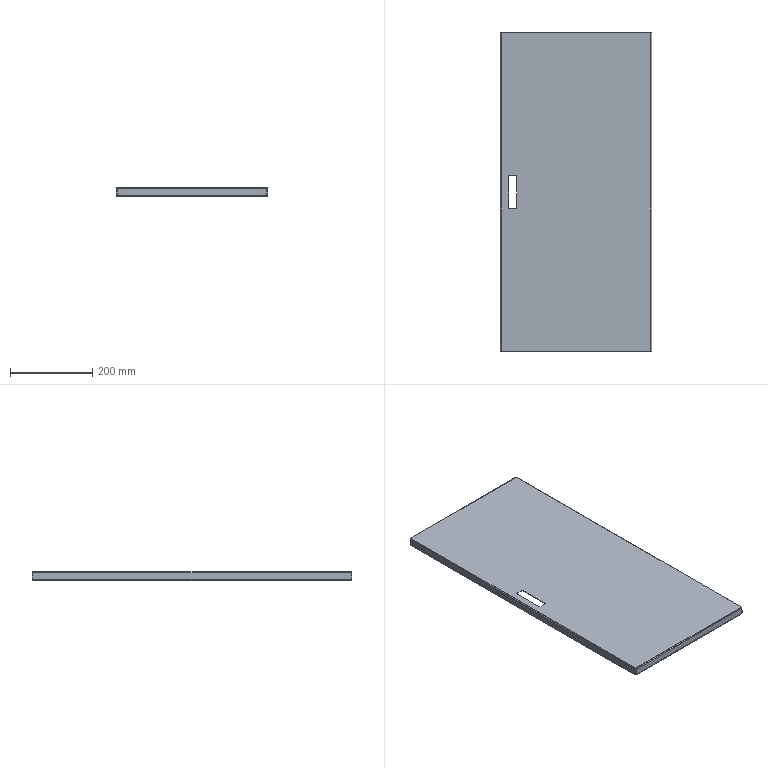Part | STEP file | X77-03008Y | 1 solid | 74 faces | box 368 x 778 x 20 mm | volume 514343 mm3 | plane 42 | spline 16 | cylinder 16 | commonest cylinder face diameters 1.473 x8 4.473 x8